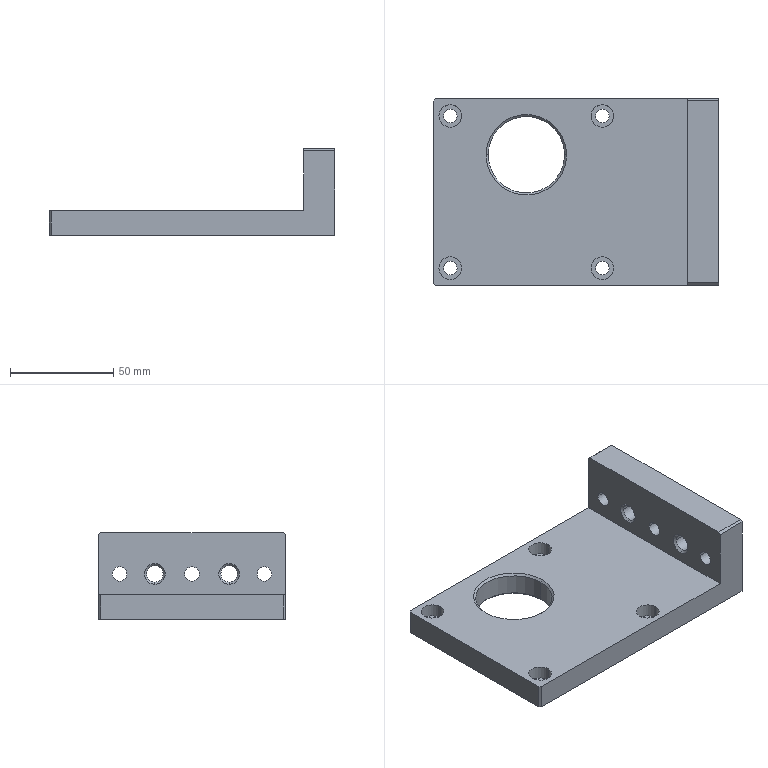Part | NX | features BREP 1 | 1 solid | 60 faces | box 138 x 90 x 42 mm | volume 169653 mm3 | cylinder 30 | plane 16 | cone 14 | commonest cylinder face diameters 6.5 x8 11 x8 7 x6 8 x4 5 x2 37 x2